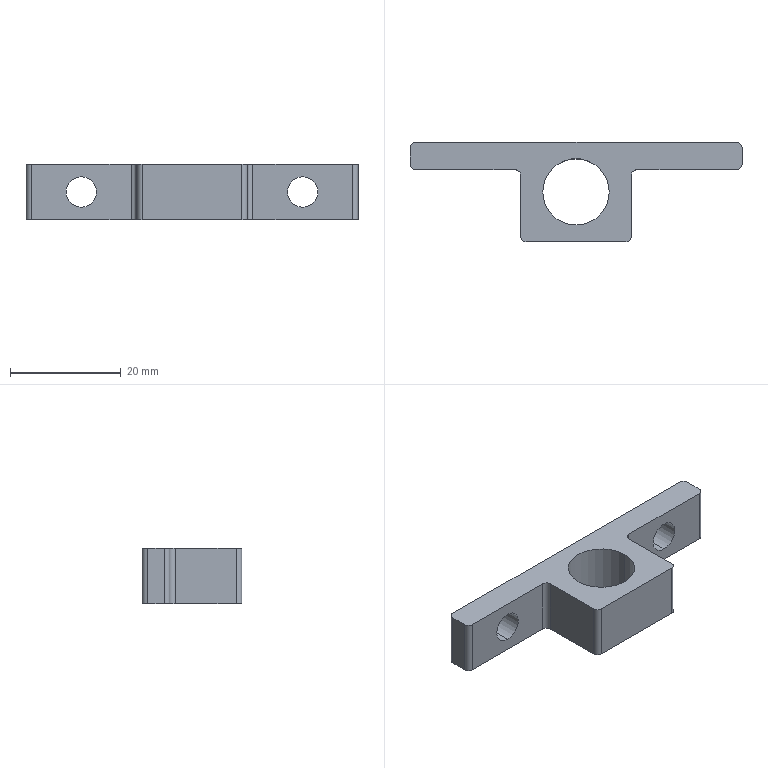Part | STEP file | Flat conveyor mechanism-CN2500x400-111-102 | 1 solid | 24 faces | box 60 x 18 x 10 mm | volume 4223 mm3 | cylinder 14 | plane 10 | commonest cylinder face diameters 2 x8 5.5 x4 12 x2
STEP:
#1=CARTESIAN_POINT('',(50.,11.,2.25));
#2=VERTEX_POINT('',#1);
#3=CARTESIAN_POINT('',(50.,11.,7.75));
#4=VERTEX_POINT('',#3);
#5=CARTESIAN_POINT('',(50.,11.,5.));
#6=DIRECTION('',(0.,1.,0.));
#7=DIRECTION('',(-1.,0.,0.));
#8=AXIS2_PLACEMENT_3D('',#5,#6,#7);
#9=CIRCLE('',#8,2.75);
#10=EDGE_CURVE('',#2,#4,#9,.T.);
#11=ORIENTED_EDGE('',*,*,#10,.F.);
#12=CARTESIAN_POINT('',(50.,16.,2.25));
#13=VERTEX_POINT('',#12);
#14=CARTESIAN_POINT('',(50.,16.,2.25));
#15=DIRECTION('',(0.,1.,0.));
#16=VECTOR('',#15,1000.);
#17=LINE('',#14,#16);
#18=EDGE_CURVE('',#2,#13,#17,.T.);
#19=ORIENTED_EDGE('',*,*,#18,.T.);
#20=CARTESIAN_POINT('',(50.,16.,7.75));
#21=VERTEX_POINT('',#20);
#22=CARTESIAN_POINT('',(50.,16.,5.));
#23=DIRECTION('',(0.,1.,0.));
#24=DIRECTION('',(0.,0.,1.));
#25=AXIS2_PLACEMENT_3D('',#22,#23,#24);
#26=CIRCLE('',#25,2.75);
#27=EDGE_CURVE('',#13,#21,#26,.T.);
#28=ORIENTED_EDGE('',*,*,#27,.T.);
#29=CARTESIAN_POINT('',(50.,16.,7.75));
#30=DIRECTION('',(0.,1.,0.));
#31=VECTOR('',#30,1000.);
#32=LINE('',#29,#31);
#33=EDGE_CURVE('',#4,#21,#32,.T.);
#34=ORIENTED_EDGE('',*,*,#33,.F.);
#35=EDGE_LOOP('',(#11,#19,#28,#34));
#36=FACE_OUTER_BOUND('',#35,.T.);
#37=CARTESIAN_POINT('',(50.,16.,5.));
#38=DIRECTION('',(0.,1.,0.));
#39=DIRECTION('',(0.,0.,1.));
#40=AXIS2_PLACEMENT_3D('',#37,#38,#39);
#41=CYLINDRICAL_SURFACE('',#40,2.75);
#42=ADVANCED_FACE('',(#36),#41,.F.);
#43=CARTESIAN_POINT('',(10.,11.,2.25));
#44=VERTEX_POINT('',#43);
#45=CARTESIAN_POINT('',(10.,11.,7.75));
#46=VERTEX_POINT('',#45);
#47=CARTESIAN_POINT('',(10.,11.,5.));
#48=DIRECTION('',(0.,1.,0.));
#49=DIRECTION('',(-1.,0.,0.));
#50=AXIS2_PLACEMENT_3D('',#47,#48,#49);
#51=CIRCLE('',#50,2.75);
#52=EDGE_CURVE('',#44,#46,#51,.T.);
#53=ORIENTED_EDGE('',*,*,#52,.F.);
#54=CARTESIAN_POINT('',(10.,16.,2.25));
#55=VERTEX_POINT('',#54);
#56=CARTESIAN_POINT('',(10.,16.,2.25));
#57=DIRECTION('',(0.,1.,0.));
#58=VECTOR('',#57,1000.);
#59=LINE('',#56,#58);
#60=EDGE_CURVE('',#44,#55,#59,.T.);
#61=ORIENTED_EDGE('',*,*,#60,.T.);
#62=CARTESIAN_POINT('',(10.,16.,7.75));
#63=VERTEX_POINT('',#62);
#64=CARTESIAN_POINT('',(10.,16.,5.));
#65=DIRECTION('',(0.,1.,0.));
#66=DIRECTION('',(0.,0.,1.));
#67=AXIS2_PLACEMENT_3D('',#64,#65,#66);
#68=CIRCLE('',#67,2.75);
#69=EDGE_CURVE('',#55,#63,#68,.T.);
#70=ORIENTED_EDGE('',*,*,#69,.T.);
#71=CARTESIAN_POINT('',(10.,16.,7.75));
#72=DIRECTION('',(0.,1.,0.));
#73=VECTOR('',#72,1000.);
#74=LINE('',#71,#73);
#75=EDGE_CURVE('',#46,#63,#74,.T.);
#76=ORIENTED_EDGE('',*,*,#75,.F.);
#77=EDGE_LOOP('',(#53,#61,#70,#76));
#78=FACE_OUTER_BOUND('',#77,.T.);
#79=CARTESIAN_POINT('',(10.,16.,5.));
#80=DIRECTION('',(0.,1.,0.));
#81=DIRECTION('',(0.,0.,1.));
#82=AXIS2_PLACEMENT_3D('',#79,#80,#81);
#83=CYLINDRICAL_SURFACE('',#82,2.75);
#84=ADVANCED_FACE('',(#78),#83,.F.);
#85=CARTESIAN_POINT('',(24.,7.,10.));
#86=VERTEX_POINT('',#85);
#87=CARTESIAN_POINT('',(36.,7.,10.));
#88=VERTEX_POINT('',#87);
#89=CARTESIAN_POINT('',(30.,7.,10.));
#90=DIRECTION('',(0.,0.,1.));
#91=DIRECTION('',(1.,0.,0.));
#92=AXIS2_PLACEMENT_3D('',#89,#90,#91);
#93=CIRCLE('',#92,6.);
#94=EDGE_CURVE('',#86,#88,#93,.T.);
#95=ORIENTED_EDGE('',*,*,#94,.T.);
#96=CARTESIAN_POINT('',(36.,7.,0.));
#97=VERTEX_POINT('',#96);
#98=CARTESIAN_POINT('',(36.,7.,10.));
#99=DIRECTION('',(0.,0.,-1.));
#100=VECTOR('',#99,1000.);
#101=LINE('',#98,#100);
#102=EDGE_CURVE('',#88,#97,#101,.T.);
#103=ORIENTED_EDGE('',*,*,#102,.T.);
#104=CARTESIAN_POINT('',(24.,7.,0.));
#105=VERTEX_POINT('',#104);
#106=CARTESIAN_POINT('',(30.,7.,0.));
#107=DIRECTION('',(0.,0.,1.));
#108=DIRECTION('',(1.,0.,0.));
#109=AXIS2_PLACEMENT_3D('',#106,#107,#108);
#110=CIRCLE('',#109,6.);
#111=EDGE_CURVE('',#105,#97,#110,.T.);
#112=ORIENTED_EDGE('',*,*,#111,.F.);
#113=CARTESIAN_POINT('',(24.,7.,10.));
#114=DIRECTION('',(0.,0.,-1.));
#115=VECTOR('',#114,1000.);
#116=LINE('',#113,#115);
#117=EDGE_CURVE('',#86,#105,#116,.T.);
#118=ORIENTED_EDGE('',*,*,#117,.F.);
#119=EDGE_LOOP('',(#95,#103,#112,#118));
#120=FACE_OUTER_BOUND('',#119,.T.);
#121=CARTESIAN_POINT('',(30.,7.,10.));
#122=DIRECTION('',(0.,0.,-1.));
#123=DIRECTION('',(-1.,0.,0.));
#124=AXIS2_PLACEMENT_3D('',#121,#122,#123);
#125=CYLINDRICAL_SURFACE('',#124,6.);
#126=ADVANCED_FACE('',(#120),#125,.F.);
#127=CARTESIAN_POINT('',(0.,12.,10.));
#128=VERTEX_POINT('',#127);
#129=CARTESIAN_POINT('',(1.,11.,10.));
#130=VERTEX_POINT('',#129);
#131=CARTESIAN_POINT('',(1.,12.,10.));
#132=DIRECTION('',(0.,0.,1.));
#133=DIRECTION('',(-1.,0.,0.));
#134=AXIS2_PLACEMENT_3D('',#131,#132,#133);
#135=CIRCLE('',#134,1.);
#136=EDGE_CURVE('',#128,#130,#135,.T.);
#137=ORIENTED_EDGE('',*,*,#136,.T.);
#138=CARTESIAN_POINT('',(19.,11.,10.));
#139=VERTEX_POINT('',#138);
#140=CARTESIAN_POINT('',(1.,11.,10.));
#141=DIRECTION('',(1.,0.,0.));
#142=VECTOR('',#141,1000.);
#143=LINE('',#140,#142);
#144=EDGE_CURVE('',#130,#139,#143,.T.);
#145=ORIENTED_EDGE('',*,*,#144,.T.);
#146=CARTESIAN_POINT('',(20.,10.,10.));
#147=VERTEX_POINT('',#146);
#148=CARTESIAN_POINT('',(19.,10.,10.));
#149=DIRECTION('',(0.,0.,-1.));
#150=DIRECTION('',(-1.,0.,0.));
#151=AXIS2_PLACEMENT_3D('',#148,#149,#150);
#152=CIRCLE('',#151,1.);
#153=EDGE_CURVE('',#139,#147,#152,.T.);
#154=ORIENTED_EDGE('',*,*,#153,.T.);
#155=CARTESIAN_POINT('',(20.,-1.,10.));
#156=VERTEX_POINT('',#155);
#157=CARTESIAN_POINT('',(20.,10.,10.));
#158=DIRECTION('',(0.,-1.,0.));
#159=VECTOR('',#158,1000.);
#160=LINE('',#157,#159);
#161=EDGE_CURVE('',#147,#156,#160,.T.);
#162=ORIENTED_EDGE('',*,*,#161,.T.);
#163=CARTESIAN_POINT('',(21.,-2.,10.));
#164=VERTEX_POINT('',#163);
#165=CARTESIAN_POINT('',(21.,-1.,10.));
#166=DIRECTION('',(0.,0.,1.));
#167=DIRECTION('',(1.,0.,0.));
#168=AXIS2_PLACEMENT_3D('',#165,#166,#167);
#169=CIRCLE('',#168,1.);
#170=EDGE_CURVE('',#156,#164,#169,.T.);
#171=ORIENTED_EDGE('',*,*,#170,.T.);
#172=CARTESIAN_POINT('',(39.,-2.,10.));
#173=VERTEX_POINT('',#172);
#174=CARTESIAN_POINT('',(21.,-2.,10.));
#175=DIRECTION('',(1.,0.,0.));
#176=VECTOR('',#175,1000.);
#177=LINE('',#174,#176);
#178=EDGE_CURVE('',#164,#173,#177,.T.);
#179=ORIENTED_EDGE('',*,*,#178,.T.);
#180=CARTESIAN_POINT('',(40.,-1.,10.));
#181=VERTEX_POINT('',#180);
#182=CARTESIAN_POINT('',(39.,-1.,10.));
#183=DIRECTION('',(0.,0.,1.));
#184=DIRECTION('',(-1.,0.,0.));
#185=AXIS2_PLACEMENT_3D('',#182,#183,#184);
#186=CIRCLE('',#185,1.);
#187=EDGE_CURVE('',#173,#181,#186,.T.);
#188=ORIENTED_EDGE('',*,*,#187,.T.);
#189=CARTESIAN_POINT('',(40.,10.,10.));
#190=VERTEX_POINT('',#189);
#191=CARTESIAN_POINT('',(40.,10.,10.));
#192=DIRECTION('',(0.,1.,0.));
#193=VECTOR('',#192,1000.);
#194=LINE('',#191,#193);
#195=EDGE_CURVE('',#181,#190,#194,.T.);
#196=ORIENTED_EDGE('',*,*,#195,.T.);
#197=CARTESIAN_POINT('',(41.,11.,10.));
#198=VERTEX_POINT('',#197);
#199=CARTESIAN_POINT('',(41.,10.,10.));
#200=DIRECTION('',(0.,0.,-1.));
#201=DIRECTION('',(1.,0.,0.));
#202=AXIS2_PLACEMENT_3D('',#199,#200,#201);
#203=CIRCLE('',#202,1.);
#204=EDGE_CURVE('',#190,#198,#203,.T.);
#205=ORIENTED_EDGE('',*,*,#204,.T.);
#206=CARTESIAN_POINT('',(59.,11.,10.));
#207=VERTEX_POINT('',#206);
#208=CARTESIAN_POINT('',(59.,11.,10.));
#209=DIRECTION('',(1.,0.,0.));
#210=VECTOR('',#209,1000.);
#211=LINE('',#208,#210);
#212=EDGE_CURVE('',#198,#207,#211,.T.);
#213=ORIENTED_EDGE('',*,*,#212,.T.);
#214=CARTESIAN_POINT('',(60.,12.,10.));
#215=VERTEX_POINT('',#214);
#216=CARTESIAN_POINT('',(59.,12.,10.));
#217=DIRECTION('',(0.,0.,1.));
#218=DIRECTION('',(1.,0.,0.));
#219=AXIS2_PLACEMENT_3D('',#216,#217,#218);
#220=CIRCLE('',#219,1.);
#221=EDGE_CURVE('',#207,#215,#220,.T.);
#222=ORIENTED_EDGE('',*,*,#221,.T.);
#223=CARTESIAN_POINT('',(60.,15.,10.));
#224=VERTEX_POINT('',#223);
#225=CARTESIAN_POINT('',(60.,12.,10.));
#226=DIRECTION('',(0.,1.,0.));
#227=VECTOR('',#226,1000.);
#228=LINE('',#225,#227);
#229=EDGE_CURVE('',#215,#224,#228,.T.);
#230=ORIENTED_EDGE('',*,*,#229,.T.);
#231=CARTESIAN_POINT('',(59.,16.,10.));
#232=VERTEX_POINT('',#231);
#233=CARTESIAN_POINT('',(59.,15.,10.));
#234=DIRECTION('',(0.,0.,1.));
#235=DIRECTION('',(-1.,0.,0.));
#236=AXIS2_PLACEMENT_3D('',#233,#234,#235);
#237=CIRCLE('',#236,1.);
#238=EDGE_CURVE('',#224,#232,#237,.T.);
#239=ORIENTED_EDGE('',*,*,#238,.T.);
#240=CARTESIAN_POINT('',(1.,16.,10.));
#241=VERTEX_POINT('',#240);
#242=CARTESIAN_POINT('',(1.,16.,10.));
#243=DIRECTION('',(-1.,0.,0.));
#244=VECTOR('',#243,1000.);
#245=LINE('',#242,#244);
#246=EDGE_CURVE('',#232,#241,#245,.T.);
#247=ORIENTED_EDGE('',*,*,#246,.T.);
#248=CARTESIAN_POINT('',(0.,15.,10.));
#249=VERTEX_POINT('',#248);
#250=CARTESIAN_POINT('',(1.,15.,10.));
#251=DIRECTION('',(0.,0.,1.));
#252=DIRECTION('',(-1.,0.,0.));
#253=AXIS2_PLACEMENT_3D('',#250,#251,#252);
#254=CIRCLE('',#253,1.);
#255=EDGE_CURVE('',#241,#249,#254,.T.);
#256=ORIENTED_EDGE('',*,*,#255,.T.);
#257=CARTESIAN_POINT('',(0.,12.,10.));
#258=DIRECTION('',(0.,-1.,0.));
#259=VECTOR('',#258,1000.);
#260=LINE('',#257,#259);
#261=EDGE_CURVE('',#249,#128,#260,.T.);
#262=ORIENTED_EDGE('',*,*,#261,.T.);
#263=EDGE_LOOP('',(#137,#145,#154,#162,#171,#179,#188,#196,#205,#213,#222,#230,#239,#247,#256,#262));
#264=FACE_OUTER_BOUND('',#263,.T.);
#265=ORIENTED_EDGE('',*,*,#94,.F.);
#266=CARTESIAN_POINT('',(30.,7.,10.));
#267=DIRECTION('',(0.,0.,1.));
#268=DIRECTION('',(1.,0.,0.));
#269=AXIS2_PLACEMENT_3D('',#266,#267,#268);
#270=CIRCLE('',#269,6.);
#271=EDGE_CURVE('',#88,#86,#270,.T.);
#272=ORIENTED_EDGE('',*,*,#271,.F.);
#273=EDGE_LOOP('',(#265,#272));
#274=FACE_BOUND('',#273,.T.);
#275=CARTESIAN_POINT('',(1.,12.,10.));
#276=DIRECTION('',(0.,0.,-1.));
#277=DIRECTION('',(-1.,0.,0.));
#278=AXIS2_PLACEMENT_3D('',#275,#276,#277);
#279=PLANE('',#278);
#280=ADVANCED_FACE('',(#264,#274),#279,.F.);
#281=CARTESIAN_POINT('',(0.,12.,0.));
#282=VERTEX_POINT('',#281);
#283=CARTESIAN_POINT('',(1.,11.,0.));
#284=VERTEX_POINT('',#283);
#285=CARTESIAN_POINT('',(1.,12.,0.));
#286=DIRECTION('',(0.,0.,1.));
#287=DIRECTION('',(-1.,0.,0.));
#288=AXIS2_PLACEMENT_3D('',#285,#286,#287);
#289=CIRCLE('',#288,1.);
#290=EDGE_CURVE('',#282,#284,#289,.T.);
#291=ORIENTED_EDGE('',*,*,#290,.F.);
#292=CARTESIAN_POINT('',(0.,15.,0.));
#293=VERTEX_POINT('',#292);
#294=CARTESIAN_POINT('',(0.,12.,0.));
#295=DIRECTION('',(0.,-1.,0.));
#296=VECTOR('',#295,1000.);
#297=LINE('',#294,#296);
#298=EDGE_CURVE('',#293,#282,#297,.T.);
#299=ORIENTED_EDGE('',*,*,#298,.F.);
#300=CARTESIAN_POINT('',(1.,16.,0.));
#301=VERTEX_POINT('',#300);
#302=CARTESIAN_POINT('',(1.,15.,0.));
#303=DIRECTION('',(0.,0.,1.));
#304=DIRECTION('',(-1.,0.,0.));
#305=AXIS2_PLACEMENT_3D('',#302,#303,#304);
#306=CIRCLE('',#305,1.);
#307=EDGE_CURVE('',#301,#293,#306,.T.);
#308=ORIENTED_EDGE('',*,*,#307,.F.);
#309=CARTESIAN_POINT('',(59.,16.,0.));
#310=VERTEX_POINT('',#309);
#311=CARTESIAN_POINT('',(1.,16.,0.));
#312=DIRECTION('',(-1.,0.,0.));
#313=VECTOR('',#312,1000.);
#314=LINE('',#311,#313);
#315=EDGE_CURVE('',#310,#301,#314,.T.);
#316=ORIENTED_EDGE('',*,*,#315,.F.);
#317=CARTESIAN_POINT('',(60.,15.,0.));
#318=VERTEX_POINT('',#317);
#319=CARTESIAN_POINT('',(59.,15.,0.));
#320=DIRECTION('',(0.,0.,1.));
#321=DIRECTION('',(-1.,0.,0.));
#322=AXIS2_PLACEMENT_3D('',#319,#320,#321);
#323=CIRCLE('',#322,1.);
#324=EDGE_CURVE('',#318,#310,#323,.T.);
#325=ORIENTED_EDGE('',*,*,#324,.F.);
#326=CARTESIAN_POINT('',(60.,12.,0.));
#327=VERTEX_POINT('',#326);
#328=CARTESIAN_POINT('',(60.,12.,0.));
#329=DIRECTION('',(0.,1.,0.));
#330=VECTOR('',#329,1000.);
#331=LINE('',#328,#330);
#332=EDGE_CURVE('',#327,#318,#331,.T.);
#333=ORIENTED_EDGE('',*,*,#332,.F.);
#334=CARTESIAN_POINT('',(59.,11.,0.));
#335=VERTEX_POINT('',#334);
#336=CARTESIAN_POINT('',(59.,12.,0.));
#337=DIRECTION('',(0.,0.,1.));
#338=DIRECTION('',(1.,0.,0.));
#339=AXIS2_PLACEMENT_3D('',#336,#337,#338);
#340=CIRCLE('',#339,1.);
#341=EDGE_CURVE('',#335,#327,#340,.T.);
#342=ORIENTED_EDGE('',*,*,#341,.F.);
#343=CARTESIAN_POINT('',(41.,11.,0.));
#344=VERTEX_POINT('',#343);
#345=CARTESIAN_POINT('',(59.,11.,0.));
#346=DIRECTION('',(1.,0.,0.));
#347=VECTOR('',#346,1000.);
#348=LINE('',#345,#347);
#349=EDGE_CURVE('',#344,#335,#348,.T.);
#350=ORIENTED_EDGE('',*,*,#349,.F.);
#351=CARTESIAN_POINT('',(40.,10.,0.));
#352=VERTEX_POINT('',#351);
#353=CARTESIAN_POINT('',(41.,10.,0.));
#354=DIRECTION('',(0.,0.,-1.));
#355=DIRECTION('',(1.,0.,0.));
#356=AXIS2_PLACEMENT_3D('',#353,#354,#355);
#357=CIRCLE('',#356,1.);
#358=EDGE_CURVE('',#352,#344,#357,.T.);
#359=ORIENTED_EDGE('',*,*,#358,.F.);
#360=CARTESIAN_POINT('',(40.,-1.,0.));
#361=VERTEX_POINT('',#360);
#362=CARTESIAN_POINT('',(40.,10.,0.));
#363=DIRECTION('',(0.,1.,0.));
#364=VECTOR('',#363,1000.);
#365=LINE('',#362,#364);
#366=EDGE_CURVE('',#361,#352,#365,.T.);
#367=ORIENTED_EDGE('',*,*,#366,.F.);
#368=CARTESIAN_POINT('',(39.,-2.,0.));
#369=VERTEX_POINT('',#368);
#370=CARTESIAN_POINT('',(39.,-1.,0.));
#371=DIRECTION('',(0.,0.,1.));
#372=DIRECTION('',(-1.,0.,0.));
#373=AXIS2_PLACEMENT_3D('',#370,#371,#372);
#374=CIRCLE('',#373,1.);
#375=EDGE_CURVE('',#369,#361,#374,.T.);
#376=ORIENTED_EDGE('',*,*,#375,.F.);
#377=CARTESIAN_POINT('',(21.,-2.,0.));
#378=VERTEX_POINT('',#377);
#379=CARTESIAN_POINT('',(21.,-2.,0.));
#380=DIRECTION('',(1.,0.,0.));
#381=VECTOR('',#380,1000.);
#382=LINE('',#379,#381);
#383=EDGE_CURVE('',#378,#369,#382,.T.);
#384=ORIENTED_EDGE('',*,*,#383,.F.);
#385=CARTESIAN_POINT('',(20.,-1.,0.));
#386=VERTEX_POINT('',#385);
#387=CARTESIAN_POINT('',(21.,-1.,0.));
#388=DIRECTION('',(0.,0.,1.));
#389=DIRECTION('',(1.,0.,0.));
#390=AXIS2_PLACEMENT_3D('',#387,#388,#389);
#391=CIRCLE('',#390,1.);
#392=EDGE_CURVE('',#386,#378,#391,.T.);
#393=ORIENTED_EDGE('',*,*,#392,.F.);
#394=CARTESIAN_POINT('',(20.,10.,0.));
#395=VERTEX_POINT('',#394);
#396=CARTESIAN_POINT('',(20.,10.,0.));
#397=DIRECTION('',(0.,-1.,0.));
#398=VECTOR('',#397,1000.);
#399=LINE('',#396,#398);
#400=EDGE_CURVE('',#395,#386,#399,.T.);
#401=ORIENTED_EDGE('',*,*,#400,.F.);
#402=CARTESIAN_POINT('',(19.,11.,0.));
#403=VERTEX_POINT('',#402);
#404=CARTESIAN_POINT('',(19.,10.,0.));
#405=DIRECTION('',(0.,0.,-1.));
#406=DIRECTION('',(-1.,0.,0.));
#407=AXIS2_PLACEMENT_3D('',#404,#405,#406);
#408=CIRCLE('',#407,1.);
#409=EDGE_CURVE('',#403,#395,#408,.T.);
#410=ORIENTED_EDGE('',*,*,#409,.F.);
#411=CARTESIAN_POINT('',(1.,11.,0.));
#412=DIRECTION('',(1.,0.,0.));
#413=VECTOR('',#412,1000.);
#414=LINE('',#411,#413);
#415=EDGE_CURVE('',#284,#403,#414,.T.);
#416=ORIENTED_EDGE('',*,*,#415,.F.);
#417=EDGE_LOOP('',(#291,#299,#308,#316,#325,#333,#342,#350,#359,#367,#376,#384,#393,#401,#410,#416));
#418=FACE_OUTER_BOUND('',#417,.T.);
#419=ORIENTED_EDGE('',*,*,#111,.T.);
#420=CARTESIAN_POINT('',(30.,7.,0.));
#421=DIRECTION('',(0.,0.,1.));
#422=DIRECTION('',(1.,0.,0.));
#423=AXIS2_PLACEMENT_3D('',#420,#421,#422);
#424=CIRCLE('',#423,6.);
#425=EDGE_CURVE('',#97,#105,#424,.T.);
#426=ORIENTED_EDGE('',*,*,#425,.T.);
#427=EDGE_LOOP('',(#419,#426));
#428=FACE_BOUND('',#427,.T.);
#429=CARTESIAN_POINT('',(1.,12.,0.));
#430=DIRECTION('',(0.,0.,-1.));
#431=DIRECTION('',(-1.,0.,0.));
#432=AXIS2_PLACEMENT_3D('',#429,#430,#431);
#433=PLANE('',#432);
#434=ADVANCED_FACE('',(#418,#428),#433,.T.);
#435=ORIENTED_EDGE('',*,*,#290,.T.);
#436=CARTESIAN_POINT('',(1.,11.,10.));
#437=DIRECTION('',(0.,0.,-1.));
#438=VECTOR('',#437,1000.);
#439=LINE('',#436,#438);
#440=EDGE_CURVE('',#130,#284,#439,.T.);
#441=ORIENTED_EDGE('',*,*,#440,.F.);
#442=ORIENTED_EDGE('',*,*,#136,.F.);
#443=CARTESIAN_POINT('',(0.,12.,10.));
#444=DIRECTION('',(0.,0.,-1.));
#445=VECTOR('',#444,1000.);
#446=LINE('',#443,#445);
#447=EDGE_CURVE('',#128,#282,#446,.T.);
#448=ORIENTED_EDGE('',*,*,#447,.T.);
#449=EDGE_LOOP('',(#435,#441,#442,#448));
#450=FACE_OUTER_BOUND('',#449,.T.);
#451=CARTESIAN_POINT('',(1.,12.,10.));
#452=DIRECTION('',(0.,0.,-1.));
#453=DIRECTION('',(-1.,0.,0.));
#454=AXIS2_PLACEMENT_3D('',#451,#452,#453);
#455=CYLINDRICAL_SURFACE('',#454,1.);
#456=ADVANCED_FACE('',(#450),#455,.T.);
#457=CARTESIAN_POINT('',(10.,11.,5.));
#458=DIRECTION('',(0.,1.,0.));
#459=DIRECTION('',(-1.,0.,0.));
#460=AXIS2_PLACEMENT_3D('',#457,#458,#459);
#461=CIRCLE('',#460,2.75);
#462=EDGE_CURVE('',#46,#44,#461,.T.);
#463=ORIENTED_EDGE('',*,*,#462,.T.);
#464=ORIENTED_EDGE('',*,*,#52,.T.);
#465=EDGE_LOOP('',(#463,#464));
#466=FACE_BOUND('',#465,.T.);
#467=ORIENTED_EDGE('',*,*,#415,.T.);
#468=CARTESIAN_POINT('',(19.,11.,10.));
#469=DIRECTION('',(0.,0.,-1.));
#470=VECTOR('',#469,1000.);
#471=LINE('',#468,#470);
#472=EDGE_CURVE('',#139,#403,#471,.T.);
#473=ORIENTED_EDGE('',*,*,#472,.F.);
#474=ORIENTED_EDGE('',*,*,#144,.F.);
#475=ORIENTED_EDGE('',*,*,#440,.T.);
#476=EDGE_LOOP('',(#467,#473,#474,#475));
#477=FACE_OUTER_BOUND('',#476,.T.);
#478=CARTESIAN_POINT('',(1.,11.,10.));
#479=DIRECTION('',(0.,1.,0.));
#480=DIRECTION('',(-1.,0.,0.));
#481=AXIS2_PLACEMENT_3D('',#478,#479,#480);
#482=PLANE('',#481);
#483=ADVANCED_FACE('',(#466,#477),#482,.F.);
#484=ORIENTED_EDGE('',*,*,#409,.T.);
#485=CARTESIAN_POINT('',(20.,10.,10.));
#486=DIRECTION('',(0.,0.,-1.));
#487=VECTOR('',#486,1000.);
#488=LINE('',#485,#487);
#489=EDGE_CURVE('',#147,#395,#488,.T.);
#490=ORIENTED_EDGE('',*,*,#489,.F.);
#491=ORIENTED_EDGE('',*,*,#153,.F.);
#492=ORIENTED_EDGE('',*,*,#472,.T.);
#493=EDGE_LOOP('',(#484,#490,#491,#492));
#494=FACE_OUTER_BOUND('',#493,.T.);
#495=CARTESIAN_POINT('',(19.,10.,10.));
#496=DIRECTION('',(0.,0.,-1.));
#497=DIRECTION('',(-1.,0.,0.));
#498=AXIS2_PLACEMENT_3D('',#495,#496,#497);
#499=CYLINDRICAL_SURFACE('',#498,1.);
#500=ADVANCED_FACE('',(#494),#499,.F.);
#501=ORIENTED_EDGE('',*,*,#400,.T.);
#502=CARTESIAN_POINT('',(20.,-1.,10.));
#503=DIRECTION('',(0.,0.,-1.));
#504=VECTOR('',#503,1000.);
#505=LINE('',#502,#504);
#506=EDGE_CURVE('',#156,#386,#505,.T.);
#507=ORIENTED_EDGE('',*,*,#506,.F.);
#508=ORIENTED_EDGE('',*,*,#161,.F.);
#509=ORIENTED_EDGE('',*,*,#489,.T.);
#510=EDGE_LOOP('',(#501,#507,#508,#509));
#511=FACE_OUTER_BOUND('',#510,.T.);
#512=CARTESIAN_POINT('',(20.,10.,10.));
#513=DIRECTION('',(1.,0.,0.));
#514=DIRECTION('',(0.,1.,0.));
#515=AXIS2_PLACEMENT_3D('',#512,#513,#514);
#516=PLANE('',#515);
#517=ADVANCED_FACE('',(#511),#516,.F.);
#518=ORIENTED_EDGE('',*,*,#392,.T.);
#519=CARTESIAN_POINT('',(21.,-2.,10.));
#520=DIRECTION('',(0.,0.,-1.));
#521=VECTOR('',#520,1000.);
#522=LINE('',#519,#521);
#523=EDGE_CURVE('',#164,#378,#522,.T.);
#524=ORIENTED_EDGE('',*,*,#523,.F.);
#525=ORIENTED_EDGE('',*,*,#170,.F.);
#526=ORIENTED_EDGE('',*,*,#506,.T.);
#527=EDGE_LOOP('',(#518,#524,#525,#526));
#528=FACE_OUTER_BOUND('',#527,.T.);
#529=CARTESIAN_POINT('',(21.,-1.,10.));
#530=DIRECTION('',(0.,0.,-1.));
#531=DIRECTION('',(-1.,0.,0.));
#532=AXIS2_PLACEMENT_3D('',#529,#530,#531);
#533=CYLINDRICAL_SURFACE('',#532,1.);
#534=ADVANCED_FACE('',(#528),#533,.T.);
#535=ORIENTED_EDGE('',*,*,#383,.T.);
#536=CARTESIAN_POINT('',(39.,-2.,10.));
#537=DIRECTION('',(0.,0.,-1.));
#538=VECTOR('',#537,1000.);
#539=LINE('',#536,#538);
#540=EDGE_CURVE('',#173,#369,#539,.T.);
#541=ORIENTED_EDGE('',*,*,#540,.F.);
#542=ORIENTED_EDGE('',*,*,#178,.F.);
#543=ORIENTED_EDGE('',*,*,#523,.T.);
#544=EDGE_LOOP('',(#535,#541,#542,#543));
#545=FACE_OUTER_BOUND('',#544,.T.);
#546=CARTESIAN_POINT('',(21.,-2.,10.));
#547=DIRECTION('',(0.,1.,0.));
#548=DIRECTION('',(-1.,0.,0.));
#549=AXIS2_PLACEMENT_3D('',#546,#547,#548);
#550=PLANE('',#549);
#551=ADVANCED_FACE('',(#545),#550,.F.);
#552=ORIENTED_EDGE('',*,*,#375,.T.);
#553=CARTESIAN_POINT('',(40.,-1.,10.));
#554=DIRECTION('',(0.,0.,-1.));
#555=VECTOR('',#554,1000.);
#556=LINE('',#553,#555);
#557=EDGE_CURVE('',#181,#361,#556,.T.);
#558=ORIENTED_EDGE('',*,*,#557,.F.);
#559=ORIENTED_EDGE('',*,*,#187,.F.);
#560=ORIENTED_EDGE('',*,*,#540,.T.);
#561=EDGE_LOOP('',(#552,#558,#559,#560));
#562=FACE_OUTER_BOUND('',#561,.T.);
#563=CARTESIAN_POINT('',(39.,-1.,10.));
#564=DIRECTION('',(0.,0.,-1.));
#565=DIRECTION('',(-1.,0.,0.));
#566=AXIS2_PLACEMENT_3D('',#563,#564,#565);
#567=CYLINDRICAL_SURFACE('',#566,1.);
#568=ADVANCED_FACE('',(#562),#567,.T.);
#569=ORIENTED_EDGE('',*,*,#366,.T.);
#570=CARTESIAN_POINT('',(40.,10.,10.));
#571=DIRECTION('',(0.,0.,-1.));
#572=VECTOR('',#571,1000.);
#573=LINE('',#570,#572);
#574=EDGE_CURVE('',#190,#352,#573,.T.);
#575=ORIENTED_EDGE('',*,*,#574,.F.);
#576=ORIENTED_EDGE('',*,*,#195,.F.);
#577=ORIENTED_EDGE('',*,*,#557,.T.);
#578=EDGE_LOOP('',(#569,#575,#576,#577));
#579=FACE_OUTER_BOUND('',#578,.T.);
#580=CARTESIAN_POINT('',(40.,10.,10.));
#581=DIRECTION('',(-1.,0.,0.));
#582=DIRECTION('',(0.,0.,1.));
#583=AXIS2_PLACEMENT_3D('',#580,#581,#582);
#584=PLANE('',#583);
#585=ADVANCED_FACE('',(#579),#584,.F.);
#586=ORIENTED_EDGE('',*,*,#358,.T.);
#587=CARTESIAN_POINT('',(41.,11.,10.));
#588=DIRECTION('',(0.,0.,-1.));
#589=VECTOR('',#588,1000.);
#590=LINE('',#587,#589);
#591=EDGE_CURVE('',#198,#344,#590,.T.);
#592=ORIENTED_EDGE('',*,*,#591,.F.);
#593=ORIENTED_EDGE('',*,*,#204,.F.);
#594=ORIENTED_EDGE('',*,*,#574,.T.);
#595=EDGE_LOOP('',(#586,#592,#593,#594));
#596=FACE_OUTER_BOUND('',#595,.T.);
#597=CARTESIAN_POINT('',(41.,10.,10.));
#598=DIRECTION('',(0.,0.,-1.));
#599=DIRECTION('',(-1.,0.,0.));
#600=AXIS2_PLACEMENT_3D('',#597,#598,#599);
#601=CYLINDRICAL_SURFACE('',#600,1.);
#602=ADVANCED_FACE('',(#596),#601,.F.);
#603=CARTESIAN_POINT('',(50.,11.,5.));
#604=DIRECTION('',(0.,1.,0.));
#605=DIRECTION('',(-1.,0.,0.));
#606=AXIS2_PLACEMENT_3D('',#603,#604,#605);
#607=CIRCLE('',#606,2.75);
#608=EDGE_CURVE('',#4,#2,#607,.T.);
#609=ORIENTED_EDGE('',*,*,#608,.T.);
#610=ORIENTED_EDGE('',*,*,#10,.T.);
#611=EDGE_LOOP('',(#609,#610));
#612=FACE_BOUND('',#611,.T.);
#613=ORIENTED_EDGE('',*,*,#349,.T.);
#614=CARTESIAN_POINT('',(59.,11.,10.));
#615=DIRECTION('',(0.,0.,-1.));
#616=VECTOR('',#615,1000.);
#617=LINE('',#614,#616);
#618=EDGE_CURVE('',#207,#335,#617,.T.);
#619=ORIENTED_EDGE('',*,*,#618,.F.);
#620=ORIENTED_EDGE('',*,*,#212,.F.);
#621=ORIENTED_EDGE('',*,*,#591,.T.);
#622=EDGE_LOOP('',(#613,#619,#620,#621));
#623=FACE_OUTER_BOUND('',#622,.T.);
#624=CARTESIAN_POINT('',(59.,11.,10.));
#625=DIRECTION('',(0.,1.,0.));
#626=DIRECTION('',(-1.,0.,0.));
#627=AXIS2_PLACEMENT_3D('',#624,#625,#626);
#628=PLANE('',#627);
#629=ADVANCED_FACE('',(#612,#623),#628,.F.);
#630=ORIENTED_EDGE('',*,*,#341,.T.);
#631=CARTESIAN_POINT('',(60.,12.,10.));
#632=DIRECTION('',(0.,0.,-1.));
#633=VECTOR('',#632,1000.);
#634=LINE('',#631,#633);
#635=EDGE_CURVE('',#215,#327,#634,.T.);
#636=ORIENTED_EDGE('',*,*,#635,.F.);
#637=ORIENTED_EDGE('',*,*,#221,.F.);
#638=ORIENTED_EDGE('',*,*,#618,.T.);
#639=EDGE_LOOP('',(#630,#636,#637,#638));
#640=FACE_OUTER_BOUND('',#639,.T.);
#641=CARTESIAN_POINT('',(59.,12.,10.));
#642=DIRECTION('',(0.,0.,-1.));
#643=DIRECTION('',(-1.,0.,0.));
#644=AXIS2_PLACEMENT_3D('',#641,#642,#643);
#645=CYLINDRICAL_SURFACE('',#644,1.);
#646=ADVANCED_FACE('',(#640),#645,.T.);
#647=ORIENTED_EDGE('',*,*,#332,.T.);
#648=CARTESIAN_POINT('',(60.,15.,10.));
#649=DIRECTION('',(0.,0.,-1.));
#650=VECTOR('',#649,1000.);
#651=LINE('',#648,#650);
#652=EDGE_CURVE('',#224,#318,#651,.T.);
#653=ORIENTED_EDGE('',*,*,#652,.F.);
#654=ORIENTED_EDGE('',*,*,#229,.F.);
#655=ORIENTED_EDGE('',*,*,#635,.T.);
#656=EDGE_LOOP('',(#647,#653,#654,#655));
#657=FACE_OUTER_BOUND('',#656,.T.);
#658=CARTESIAN_POINT('',(60.,12.,10.));
#659=DIRECTION('',(-1.,0.,0.));
#660=DIRECTION('',(0.,-1.,0.));
#661=AXIS2_PLACEMENT_3D('',#658,#659,#660);
#662=PLANE('',#661);
#663=ADVANCED_FACE('',(#657),#662,.F.);
#664=ORIENTED_EDGE('',*,*,#324,.T.);
#665=CARTESIAN_POINT('',(59.,16.,10.));
#666=DIRECTION('',(0.,0.,-1.));
#667=VECTOR('',#666,1000.);
#668=LINE('',#665,#667);
#669=EDGE_CURVE('',#232,#310,#668,.T.);
#670=ORIENTED_EDGE('',*,*,#669,.F.);
#671=ORIENTED_EDGE('',*,*,#238,.F.);
#672=ORIENTED_EDGE('',*,*,#652,.T.);
#673=EDGE_LOOP('',(#664,#670,#671,#672));
#674=FACE_OUTER_BOUND('',#673,.T.);
#675=CARTESIAN_POINT('',(59.,15.,10.));
#676=DIRECTION('',(0.,0.,-1.));
#677=DIRECTION('',(-1.,0.,0.));
#678=AXIS2_PLACEMENT_3D('',#675,#676,#677);
#679=CYLINDRICAL_SURFACE('',#678,1.);
#680=ADVANCED_FACE('',(#674),#679,.T.);
#681=CARTESIAN_POINT('',(50.,16.,5.));
#682=DIRECTION('',(0.,1.,0.));
#683=DIRECTION('',(0.,0.,1.));
#684=AXIS2_PLACEMENT_3D('',#681,#682,#683);
#685=CIRCLE('',#684,2.75);
#686=EDGE_CURVE('',#21,#13,#685,.T.);
#687=ORIENTED_EDGE('',*,*,#686,.F.);
#688=ORIENTED_EDGE('',*,*,#27,.F.);
#689=EDGE_LOOP('',(#687,#688));
#690=FACE_BOUND('',#689,.T.);
#691=CARTESIAN_POINT('',(10.,16.,5.));
#692=DIRECTION('',(0.,1.,0.));
#693=DIRECTION('',(0.,0.,1.));
#694=AXIS2_PLACEMENT_3D('',#691,#692,#693);
#695=CIRCLE('',#694,2.75);
#696=EDGE_CURVE('',#63,#55,#695,.T.);
#697=ORIENTED_EDGE('',*,*,#696,.F.);
#698=ORIENTED_EDGE('',*,*,#69,.F.);
#699=EDGE_LOOP('',(#697,#698));
#700=FACE_BOUND('',#699,.T.);
#701=ORIENTED_EDGE('',*,*,#315,.T.);
#702=CARTESIAN_POINT('',(1.,16.,10.));
#703=DIRECTION('',(0.,0.,-1.));
#704=VECTOR('',#703,1000.);
#705=LINE('',#702,#704);
#706=EDGE_CURVE('',#241,#301,#705,.T.);
#707=ORIENTED_EDGE('',*,*,#706,.F.);
#708=ORIENTED_EDGE('',*,*,#246,.F.);
#709=ORIENTED_EDGE('',*,*,#669,.T.);
#710=EDGE_LOOP('',(#701,#707,#708,#709));
#711=FACE_OUTER_BOUND('',#710,.T.);
#712=CARTESIAN_POINT('',(1.,16.,10.));
#713=DIRECTION('',(0.,-1.,0.));
#714=DIRECTION('',(0.,0.,-1.));
#715=AXIS2_PLACEMENT_3D('',#712,#713,#714);
#716=PLANE('',#715);
#717=ADVANCED_FACE('',(#690,#700,#711),#716,.F.);
#718=ORIENTED_EDGE('',*,*,#307,.T.);
#719=CARTESIAN_POINT('',(0.,15.,10.));
#720=DIRECTION('',(0.,0.,-1.));
#721=VECTOR('',#720,1000.);
#722=LINE('',#719,#721);
#723=EDGE_CURVE('',#249,#293,#722,.T.);
#724=ORIENTED_EDGE('',*,*,#723,.F.);
#725=ORIENTED_EDGE('',*,*,#255,.F.);
#726=ORIENTED_EDGE('',*,*,#706,.T.);
#727=EDGE_LOOP('',(#718,#724,#725,#726));
#728=FACE_OUTER_BOUND('',#727,.T.);
#729=CARTESIAN_POINT('',(1.,15.,10.));
#730=DIRECTION('',(0.,0.,-1.));
#731=DIRECTION('',(-1.,0.,0.));
#732=AXIS2_PLACEMENT_3D('',#729,#730,#731);
#733=CYLINDRICAL_SURFACE('',#732,1.);
#734=ADVANCED_FACE('',(#728),#733,.T.);
#735=ORIENTED_EDGE('',*,*,#298,.T.);
#736=ORIENTED_EDGE('',*,*,#447,.F.);
#737=ORIENTED_EDGE('',*,*,#261,.F.);
#738=ORIENTED_EDGE('',*,*,#723,.T.);
#739=EDGE_LOOP('',(#735,#736,#737,#738));
#740=FACE_OUTER_BOUND('',#739,.T.);
#741=CARTESIAN_POINT('',(0.,12.,10.));
#742=DIRECTION('',(1.,0.,0.));
#743=DIRECTION('',(0.,0.,-1.));
#744=AXIS2_PLACEMENT_3D('',#741,#742,#743);
#745=PLANE('',#744);
#746=ADVANCED_FACE('',(#740),#745,.F.);
#747=ORIENTED_EDGE('',*,*,#102,.F.);
#748=ORIENTED_EDGE('',*,*,#271,.T.);
#749=ORIENTED_EDGE('',*,*,#117,.T.);
#750=ORIENTED_EDGE('',*,*,#425,.F.);
#751=EDGE_LOOP('',(#747,#748,#749,#750));
#752=FACE_OUTER_BOUND('',#751,.T.);
#753=CARTESIAN_POINT('',(30.,7.,10.));
#754=DIRECTION('',(0.,0.,-1.));
#755=DIRECTION('',(-1.,0.,0.));
#756=AXIS2_PLACEMENT_3D('',#753,#754,#755);
#757=CYLINDRICAL_SURFACE('',#756,6.);
#758=ADVANCED_FACE('',(#752),#757,.F.);
#759=ORIENTED_EDGE('',*,*,#60,.F.);
#760=ORIENTED_EDGE('',*,*,#462,.F.);
#761=ORIENTED_EDGE('',*,*,#75,.T.);
#762=ORIENTED_EDGE('',*,*,#696,.T.);
#763=EDGE_LOOP('',(#759,#760,#761,#762));
#764=FACE_OUTER_BOUND('',#763,.T.);
#765=CARTESIAN_POINT('',(10.,16.,5.));
#766=DIRECTION('',(0.,1.,0.));
#767=DIRECTION('',(0.,0.,1.));
#768=AXIS2_PLACEMENT_3D('',#765,#766,#767);
#769=CYLINDRICAL_SURFACE('',#768,2.75);
#770=ADVANCED_FACE('',(#764),#769,.F.);
#771=ORIENTED_EDGE('',*,*,#18,.F.);
#772=ORIENTED_EDGE('',*,*,#608,.F.);
#773=ORIENTED_EDGE('',*,*,#33,.T.);
#774=ORIENTED_EDGE('',*,*,#686,.T.);
#775=EDGE_LOOP('',(#771,#772,#773,#774));
#776=FACE_OUTER_BOUND('',#775,.T.);
#777=CARTESIAN_POINT('',(50.,16.,5.));
#778=DIRECTION('',(0.,1.,0.));
#779=DIRECTION('',(0.,0.,1.));
#780=AXIS2_PLACEMENT_3D('',#777,#778,#779);
#781=CYLINDRICAL_SURFACE('',#780,2.75);
#782=ADVANCED_FACE('',(#776),#781,.F.);
#783=CLOSED_SHELL('',(#42,#84,#126,#280,#434,#456,#483,#500,#517,#534,#551,#568,#585,#602,#629,#646,#663,#680,#717,#734,#746,#758,#770,#782));
#784=MANIFOLD_SOLID_BREP('',#783);
#785=CARTESIAN_POINT('',(0.,0.,0.));
#786=DIRECTION('',(0.,0.,1.));
#787=DIRECTION('',(1.,0.,0.));
#788=AXIS2_PLACEMENT_3D('',#785,#786,#787);
#789=(LENGTH_UNIT()NAMED_UNIT(*)SI_UNIT(.MILLI.,.METRE.));
#790=UNCERTAINTY_MEASURE_WITH_UNIT(LENGTH_MEASURE(0.00001),#789,'','');
#791=(NAMED_UNIT(*)PLANE_ANGLE_UNIT()SI_UNIT($,.RADIAN.));
#792=(NAMED_UNIT(*)SI_UNIT($,.STERADIAN.)SOLID_ANGLE_UNIT());
#793=(GEOMETRIC_REPRESENTATION_CONTEXT(3)GLOBAL_UNCERTAINTY_ASSIGNED_CONTEXT((#790))GLOBAL_UNIT_ASSIGNED_CONTEXT((#789,#791,#792))REPRESENTATION_CONTEXT('',''));
#794=ADVANCED_BREP_SHAPE_REPRESENTATION('',(#784,#788),#793);